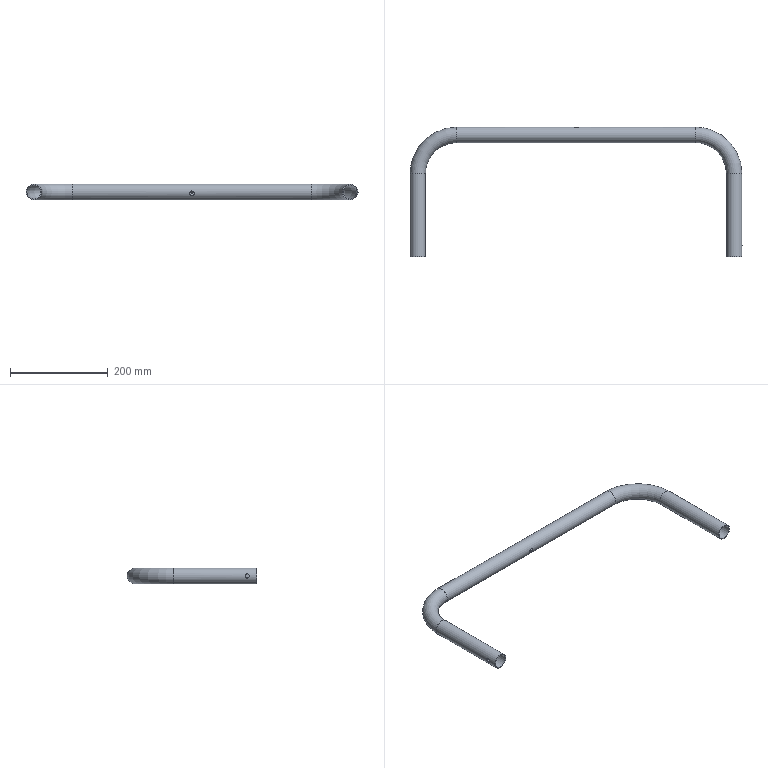Part | STEP file | 6151301 | 1 solid | 16 faces | box 679.8 x 265.9 x 31.8 mm | volume 153699 mm3 | cylinder 10 | torus 4 | plane 2 | commonest cylinder face diameters 28.8 x3 31.8 x3 8.5 x2 10 x2
STEP:
#1=CARTESIAN_POINT('',(0.,263.929,7.668));
#2=VERTEX_POINT('',#1);
#3=CARTESIAN_POINT('',(0.,263.929,7.668));
#4=CARTESIAN_POINT('',(-0.3326,263.929,7.668));
#5=CARTESIAN_POINT('',(-0.6592,263.946,7.638));
#6=CARTESIAN_POINT('',(-1.301,264.01,7.519));
#7=CARTESIAN_POINT('',(-1.62,264.058,7.429));
#8=CARTESIAN_POINT('',(-2.224,264.179,7.196));
#9=CARTESIAN_POINT('',(-2.51,264.251,7.053));
#10=CARTESIAN_POINT('',(-3.052,264.414,6.714));
#11=CARTESIAN_POINT('',(-3.307,264.505,6.518));
#12=CARTESIAN_POINT('',(-3.765,264.691,6.086));
#13=CARTESIAN_POINT('',(-3.971,264.787,5.85));
#14=CARTESIAN_POINT('',(-4.337,264.982,5.331));
#15=CARTESIAN_POINT('',(-4.491,265.078,5.056));
#16=CARTESIAN_POINT('',(-4.678,265.214,4.623));
#17=CARTESIAN_POINT('',(-4.734,265.258,4.475));
#18=CARTESIAN_POINT('',(-4.83,265.344,4.171));
#19=CARTESIAN_POINT('',(-4.871,265.386,4.015));
#20=CARTESIAN_POINT('',(-4.968,265.503,3.544));
#21=CARTESIAN_POINT('',(-5.,265.573,3.225));
#22=CARTESIAN_POINT('',(-5.,265.693,2.579));
#23=CARTESIAN_POINT('',(-4.967,265.743,2.249));
#24=CARTESIAN_POINT('',(-4.839,265.822,1.609));
#25=CARTESIAN_POINT('',(-4.744,265.85,1.297));
#26=CARTESIAN_POINT('',(-4.491,265.888,0.685));
#27=CARTESIAN_POINT('',(-4.335,265.898,0.3928));
#28=CARTESIAN_POINT('',(-3.974,265.902,-0.1551));
#29=CARTESIAN_POINT('',(-3.765,265.896,-0.4149));
#30=CARTESIAN_POINT('',(-3.304,265.877,-0.8872));
#31=CARTESIAN_POINT('',(-3.054,265.863,-1.099));
#32=CARTESIAN_POINT('',(-2.514,265.833,-1.472));
#33=CARTESIAN_POINT('',(-2.221,265.816,-1.635));
#34=CARTESIAN_POINT('',(-1.619,265.787,-1.895));
#35=CARTESIAN_POINT('',(-1.308,265.775,-1.995));
#36=CARTESIAN_POINT('',(-0.823,265.761,-2.096));
#37=CARTESIAN_POINT('',(-0.658,265.758,-2.122));
#38=CARTESIAN_POINT('',(-0.3299,265.753,-2.156));
#39=CARTESIAN_POINT('',(-0.166,265.752,-2.164));
#40=CARTESIAN_POINT('',(0.3255,265.752,-2.165));
#41=CARTESIAN_POINT('',(0.6546,265.757,-2.131));
#42=CARTESIAN_POINT('',(1.304,265.774,-1.996));
#43=CARTESIAN_POINT('',(1.616,265.787,-1.896));
#44=CARTESIAN_POINT('',(2.219,265.816,-1.636));
#45=CARTESIAN_POINT('',(2.512,265.833,-1.474));
#46=CARTESIAN_POINT('',(3.052,265.863,-1.1));
#47=CARTESIAN_POINT('',(3.303,265.877,-0.8884));
#48=CARTESIAN_POINT('',(3.765,265.896,-0.4156));
#49=CARTESIAN_POINT('',(3.973,265.902,-0.1564));
#50=CARTESIAN_POINT('',(4.334,265.898,0.3906));
#51=CARTESIAN_POINT('',(4.489,265.888,0.6818));
#52=CARTESIAN_POINT('',(4.743,265.85,1.294));
#53=CARTESIAN_POINT('',(4.838,265.822,1.607));
#54=CARTESIAN_POINT('',(4.934,265.764,2.085));
#55=CARTESIAN_POINT('',(4.959,265.741,2.246));
#56=CARTESIAN_POINT('',(4.992,265.692,2.571));
#57=CARTESIAN_POINT('',(5.,265.664,2.736));
#58=CARTESIAN_POINT('',(5.,265.574,3.222));
#59=CARTESIAN_POINT('',(4.968,265.504,3.541));
#60=CARTESIAN_POINT('',(4.839,265.347,4.168));
#61=CARTESIAN_POINT('',(4.742,265.26,4.476));
#62=CARTESIAN_POINT('',(4.491,265.078,5.055));
#63=CARTESIAN_POINT('',(4.337,264.983,5.33));
#64=CARTESIAN_POINT('',(3.972,264.788,5.849));
#65=CARTESIAN_POINT('',(3.765,264.691,6.086));
#66=CARTESIAN_POINT('',(3.307,264.505,6.518));
#67=CARTESIAN_POINT('',(3.052,264.414,6.714));
#68=CARTESIAN_POINT('',(2.511,264.252,7.053));
#69=CARTESIAN_POINT('',(2.225,264.179,7.195));
#70=CARTESIAN_POINT('',(1.621,264.059,7.429));
#71=CARTESIAN_POINT('',(1.302,264.01,7.519));
#72=CARTESIAN_POINT('',(0.6596,263.946,7.638));
#73=CARTESIAN_POINT('',(0.3326,263.929,7.668));
#74=CARTESIAN_POINT('',(0.,263.929,7.668));
#75=B_SPLINE_CURVE_WITH_KNOTS('',3,(#3,#4,#5,#6,#7,#8,#9,#10,#11,#12,#13,#14,#15,#16,#17,#18,#19,#20,#21,#22,#23,#24,#25,#26,#27,#28,#29,#30,#31,#32,#33,#34,#35,#36,#37,#38,#39,#40,#41,#42,#43,#44,#45,#46,#47,#48,#49,#50,#51,#52,#53,#54,#55,#56,#57,#58,#59,#60,#61,#62,#63,#64,#65,#66,#67,#68,#69,#70,#71,#72,#73,#74),.UNSPECIFIED.,.T.,.F.,(4,2,2,2,2,2,2,2,2,2,2,2,2,2,2,2,2,2,2,2,2,2,2,2,2,2,2,2,2,2,2,2,2,2,2,4),(0.,0.0009831,0.001966,0.002949,0.003933,0.004916,0.005899,0.00639,0.006882,0.007865,0.008848,0.009831,0.01081,0.0118,0.01278,0.01376,0.01475,0.01524,0.01573,0.01671,0.0177,0.01868,0.01966,0.02065,0.02163,0.02261,0.0231,0.0236,0.02458,0.02556,0.02654,0.02753,0.02851,0.02949,0.03048,0.03146),.UNSPECIFIED.);
#76=EDGE_CURVE('',#2,#2,#75,.T.);
#77=ORIENTED_EDGE('',*,*,#76,.T.);
#78=EDGE_LOOP('',(#77));
#79=FACE_BOUND('',#78,.T.);
#80=CARTESIAN_POINT('',(244.,250.,15.9));
#81=VERTEX_POINT('',#80);
#82=CARTESIAN_POINT('',(244.,250.,0.));
#83=DIRECTION('',(-1.,0.,0.));
#84=DIRECTION('',(0.,0.,1.));
#85=AXIS2_PLACEMENT_3D('',#82,#83,#84);
#86=CIRCLE('',#85,15.9);
#87=EDGE_CURVE('',#81,#81,#86,.T.);
#88=ORIENTED_EDGE('',*,*,#87,.T.);
#89=EDGE_LOOP('',(#88));
#90=FACE_OUTER_BOUND('',#89,.T.);
#91=CARTESIAN_POINT('',(-244.,250.,15.9));
#92=VERTEX_POINT('',#91);
#93=CARTESIAN_POINT('',(-244.,250.,0.));
#94=DIRECTION('',(-1.,0.,0.));
#95=DIRECTION('',(0.,0.,1.));
#96=AXIS2_PLACEMENT_3D('',#93,#94,#95);
#97=CIRCLE('',#96,15.9);
#98=EDGE_CURVE('',#92,#92,#97,.T.);
#99=ORIENTED_EDGE('',*,*,#98,.F.);
#100=EDGE_LOOP('',(#99));
#101=FACE_OUTER_BOUND('',#100,.T.);
#102=CARTESIAN_POINT('',(0.,234.248,2.167));
#103=VERTEX_POINT('',#102);
#104=CARTESIAN_POINT('',(0.,234.248,2.167));
#105=CARTESIAN_POINT('',(0.3326,234.248,2.167));
#106=CARTESIAN_POINT('',(0.6592,234.244,2.133));
#107=CARTESIAN_POINT('',(1.301,234.226,1.999));
#108=CARTESIAN_POINT('',(1.62,234.213,1.898));
#109=CARTESIAN_POINT('',(2.224,234.184,1.636));
#110=CARTESIAN_POINT('',(2.51,234.168,1.477));
#111=CARTESIAN_POINT('',(3.052,234.137,1.103));
#112=CARTESIAN_POINT('',(3.307,234.123,0.8869));
#113=CARTESIAN_POINT('',(3.765,234.104,0.4175));
#114=CARTESIAN_POINT('',(3.971,234.098,0.1619));
#115=CARTESIAN_POINT('',(4.337,234.102,-0.3926));
#116=CARTESIAN_POINT('',(4.491,234.112,-0.6832));
#117=CARTESIAN_POINT('',(4.678,234.14,-1.136));
#118=CARTESIAN_POINT('',(4.734,234.152,-1.29));
#119=CARTESIAN_POINT('',(4.83,234.18,-1.605));
#120=CARTESIAN_POINT('',(4.871,234.198,-1.766));
#121=CARTESIAN_POINT('',(4.968,234.256,-2.248));
#122=CARTESIAN_POINT('',(5.,234.306,-2.57));
#123=CARTESIAN_POINT('',(5.,234.425,-3.216));
#124=CARTESIAN_POINT('',(4.967,234.496,-3.542));
#125=CARTESIAN_POINT('',(4.839,234.652,-4.167));
#126=CARTESIAN_POINT('',(4.744,234.738,-4.47));
#127=CARTESIAN_POINT('',(4.491,234.922,-5.054));
#128=CARTESIAN_POINT('',(4.335,235.018,-5.33));
#129=CARTESIAN_POINT('',(3.974,235.21,-5.843));
#130=CARTESIAN_POINT('',(3.765,235.308,-6.084));
#131=CARTESIAN_POINT('',(3.304,235.495,-6.518));
#132=CARTESIAN_POINT('',(3.054,235.584,-6.711));
#133=CARTESIAN_POINT('',(2.514,235.746,-7.049));
#134=CARTESIAN_POINT('',(2.221,235.82,-7.195));
#135=CARTESIAN_POINT('',(1.619,235.941,-7.427));
#136=CARTESIAN_POINT('',(1.308,235.988,-7.515));
#137=CARTESIAN_POINT('',(0.823,236.037,-7.605));
#138=CARTESIAN_POINT('',(0.658,236.049,-7.628));
#139=CARTESIAN_POINT('',(0.3299,236.066,-7.658));
#140=CARTESIAN_POINT('',(0.166,236.07,-7.666));
#141=CARTESIAN_POINT('',(-0.3255,236.07,-7.666));
#142=CARTESIAN_POINT('',(-0.6546,236.054,-7.636));
#143=CARTESIAN_POINT('',(-1.304,235.989,-7.516));
#144=CARTESIAN_POINT('',(-1.616,235.941,-7.428));
#145=CARTESIAN_POINT('',(-2.219,235.821,-7.196));
#146=CARTESIAN_POINT('',(-2.512,235.747,-7.05));
#147=CARTESIAN_POINT('',(-3.052,235.585,-6.712));
#148=CARTESIAN_POINT('',(-3.303,235.496,-6.519));
#149=CARTESIAN_POINT('',(-3.765,235.308,-6.085));
#150=CARTESIAN_POINT('',(-3.973,235.211,-5.845));
#151=CARTESIAN_POINT('',(-4.334,235.018,-5.333));
#152=CARTESIAN_POINT('',(-4.489,234.923,-5.057));
#153=CARTESIAN_POINT('',(-4.743,234.739,-4.472));
#154=CARTESIAN_POINT('',(-4.838,234.653,-4.17));
#155=CARTESIAN_POINT('',(-4.934,234.536,-3.703));
#156=CARTESIAN_POINT('',(-4.959,234.499,-3.544));
#157=CARTESIAN_POINT('',(-4.992,234.429,-3.223));
#158=CARTESIAN_POINT('',(-5.,234.396,-3.059));
#159=CARTESIAN_POINT('',(-5.,234.306,-2.573));
#160=CARTESIAN_POINT('',(-4.968,234.257,-2.251));
#161=CARTESIAN_POINT('',(-4.839,234.178,-1.609));
#162=CARTESIAN_POINT('',(-4.742,234.15,-1.29));
#163=CARTESIAN_POINT('',(-4.491,234.112,-0.6845));
#164=CARTESIAN_POINT('',(-4.337,234.102,-0.3932));
#165=CARTESIAN_POINT('',(-3.972,234.098,0.1612));
#166=CARTESIAN_POINT('',(-3.765,234.104,0.4169));
#167=CARTESIAN_POINT('',(-3.307,234.123,0.8867));
#168=CARTESIAN_POINT('',(-3.052,234.137,1.103));
#169=CARTESIAN_POINT('',(-2.511,234.168,1.477));
#170=CARTESIAN_POINT('',(-2.225,234.184,1.636));
#171=CARTESIAN_POINT('',(-1.621,234.213,1.897));
#172=CARTESIAN_POINT('',(-1.302,234.226,1.999));
#173=CARTESIAN_POINT('',(-0.6596,234.244,2.133));
#174=CARTESIAN_POINT('',(-0.3326,234.248,2.167));
#175=CARTESIAN_POINT('',(0.,234.248,2.167));
#176=B_SPLINE_CURVE_WITH_KNOTS('',3,(#104,#105,#106,#107,#108,#109,#110,#111,#112,#113,#114,#115,#116,#117,#118,#119,#120,#121,#122,#123,#124,#125,#126,#127,#128,#129,#130,#131,#132,#133,#134,#135,#136,#137,#138,#139,#140,#141,#142,#143,#144,#145,#146,#147,#148,#149,#150,#151,#152,#153,#154,#155,#156,#157,#158,#159,#160,#161,#162,#163,#164,#165,#166,#167,#168,#169,#170,#171,#172,#173,#174,#175),.UNSPECIFIED.,.T.,.F.,(4,2,2,2,2,2,2,2,2,2,2,2,2,2,2,2,2,2,2,2,2,2,2,2,2,2,2,2,2,2,2,2,2,2,2,4),(0.,0.0009831,0.001966,0.002949,0.003933,0.004916,0.005899,0.00639,0.006882,0.007865,0.008848,0.009831,0.01081,0.0118,0.01278,0.01376,0.01475,0.01524,0.01573,0.01671,0.0177,0.01868,0.01966,0.02065,0.02163,0.02261,0.0231,0.0236,0.02458,0.02556,0.02654,0.02753,0.02851,0.02949,0.03048,0.03146),.UNSPECIFIED.);
#177=EDGE_CURVE('',#103,#103,#176,.T.);
#178=ORIENTED_EDGE('',*,*,#177,.T.);
#179=EDGE_LOOP('',(#178));
#180=FACE_BOUND('',#179,.T.);
#181=CARTESIAN_POINT('',(244.,250.,0.));
#182=DIRECTION('',(-1.,0.,0.));
#183=DIRECTION('',(0.,0.,1.));
#184=AXIS2_PLACEMENT_3D('',#181,#182,#183);
#185=CYLINDRICAL_SURFACE('',#184,15.9);
#186=ADVANCED_FACE('',(#79,#90,#101,#180),#185,.T.);
#187=CARTESIAN_POINT('',(0.,262.366,7.378));
#188=VERTEX_POINT('',#187);
#189=CARTESIAN_POINT('',(0.,262.366,7.378));
#190=CARTESIAN_POINT('',(-0.3331,262.366,7.378));
#191=CARTESIAN_POINT('',(-0.6602,262.384,7.348));
#192=CARTESIAN_POINT('',(-1.303,262.453,7.23));
#193=CARTESIAN_POINT('',(-1.621,262.505,7.141));
#194=CARTESIAN_POINT('',(-2.226,262.635,6.909));
#195=CARTESIAN_POINT('',(-2.512,262.712,6.767));
#196=CARTESIAN_POINT('',(-3.053,262.886,6.43));
#197=CARTESIAN_POINT('',(-3.307,262.982,6.235));
#198=CARTESIAN_POINT('',(-3.764,263.179,5.807));
#199=CARTESIAN_POINT('',(-3.971,263.281,5.571));
#200=CARTESIAN_POINT('',(-4.336,263.487,5.054));
#201=CARTESIAN_POINT('',(-4.49,263.586,4.781));
#202=CARTESIAN_POINT('',(-4.678,263.728,4.349));
#203=CARTESIAN_POINT('',(-4.733,263.774,4.202));
#204=CARTESIAN_POINT('',(-4.829,263.863,3.898));
#205=CARTESIAN_POINT('',(-4.87,263.906,3.742));
#206=CARTESIAN_POINT('',(-4.967,264.027,3.271));
#207=CARTESIAN_POINT('',(-5.,264.098,2.952));
#208=CARTESIAN_POINT('',(-5.,264.218,2.305));
#209=CARTESIAN_POINT('',(-4.967,264.268,1.974));
#210=CARTESIAN_POINT('',(-4.838,264.342,1.334));
#211=CARTESIAN_POINT('',(-4.743,264.367,1.02));
#212=CARTESIAN_POINT('',(-4.489,264.398,0.4061));
#213=CARTESIAN_POINT('',(-4.334,264.402,0.114));
#214=CARTESIAN_POINT('',(-3.973,264.396,-0.4354));
#215=CARTESIAN_POINT('',(-3.764,264.385,-0.6962));
#216=CARTESIAN_POINT('',(-3.304,264.354,-1.169));
#217=CARTESIAN_POINT('',(-3.054,264.335,-1.382));
#218=CARTESIAN_POINT('',(-2.515,264.294,-1.757));
#219=CARTESIAN_POINT('',(-2.222,264.272,-1.921));
#220=CARTESIAN_POINT('',(-1.621,264.234,-2.183));
#221=CARTESIAN_POINT('',(-1.309,264.218,-2.283));
#222=CARTESIAN_POINT('',(-0.8233,264.201,-2.385));
#223=CARTESIAN_POINT('',(-0.6582,264.197,-2.411));
#224=CARTESIAN_POINT('',(-0.3301,264.191,-2.446));
#225=CARTESIAN_POINT('',(-0.001961,264.188,-2.463));
#226=CARTESIAN_POINT('',(0.3261,264.191,-2.446));
#227=CARTESIAN_POINT('',(0.6541,264.197,-2.412));
#228=CARTESIAN_POINT('',(0.819,264.201,-2.386));
#229=CARTESIAN_POINT('',(1.306,264.218,-2.284));
#230=CARTESIAN_POINT('',(1.618,264.234,-2.184));
#231=CARTESIAN_POINT('',(2.222,264.272,-1.921));
#232=CARTESIAN_POINT('',(2.514,264.294,-1.758));
#233=CARTESIAN_POINT('',(3.053,264.335,-1.383));
#234=CARTESIAN_POINT('',(3.304,264.354,-1.17));
#235=CARTESIAN_POINT('',(3.766,264.385,-0.6944));
#236=CARTESIAN_POINT('',(3.973,264.396,-0.4358));
#237=CARTESIAN_POINT('',(4.333,264.402,0.1125));
#238=CARTESIAN_POINT('',(4.489,264.398,0.4062));
#239=CARTESIAN_POINT('',(4.742,264.367,1.018));
#240=CARTESIAN_POINT('',(4.838,264.342,1.331));
#241=CARTESIAN_POINT('',(4.967,264.268,1.971));
#242=CARTESIAN_POINT('',(5.,264.219,2.302));
#243=CARTESIAN_POINT('',(5.,264.099,2.95));
#244=CARTESIAN_POINT('',(4.968,264.028,3.269));
#245=CARTESIAN_POINT('',(4.871,263.907,3.74));
#246=CARTESIAN_POINT('',(4.83,263.864,3.896));
#247=CARTESIAN_POINT('',(4.734,263.775,4.2));
#248=CARTESIAN_POINT('',(4.678,263.729,4.348));
#249=CARTESIAN_POINT('',(4.49,263.587,4.781));
#250=CARTESIAN_POINT('',(4.335,263.486,5.057));
#251=CARTESIAN_POINT('',(3.97,263.281,5.572));
#252=CARTESIAN_POINT('',(3.764,263.179,5.807));
#253=CARTESIAN_POINT('',(3.306,262.982,6.237));
#254=CARTESIAN_POINT('',(3.05,262.885,6.432));
#255=CARTESIAN_POINT('',(2.511,262.712,6.767));
#256=CARTESIAN_POINT('',(2.225,262.635,6.909));
#257=CARTESIAN_POINT('',(1.771,262.538,7.083));
#258=CARTESIAN_POINT('',(1.615,262.508,7.135));
#259=CARTESIAN_POINT('',(1.3,262.458,7.223));
#260=CARTESIAN_POINT('',(1.141,262.436,7.26));
#261=CARTESIAN_POINT('',(0.6602,262.384,7.348));
#262=CARTESIAN_POINT('',(0.3331,262.366,7.378));
#263=CARTESIAN_POINT('',(0.,262.366,7.378));
#264=B_SPLINE_CURVE_WITH_KNOTS('',3,(#189,#190,#191,#192,#193,#194,#195,#196,#197,#198,#199,#200,#201,#202,#203,#204,#205,#206,#207,#208,#209,#210,#211,#212,#213,#214,#215,#216,#217,#218,#219,#220,#221,#222,#223,#224,#225,#226,#227,#228,#229,#230,#231,#232,#233,#234,#235,#236,#237,#238,#239,#240,#241,#242,#243,#244,#245,#246,#247,#248,#249,#250,#251,#252,#253,#254,#255,#256,#257,#258,#259,#260,#261,#262,#263),.UNSPECIFIED.,.T.,.F.,(4,2,2,2,2,2,2,2,2,2,2,2,2,2,2,2,2,2,1,2,2,2,2,2,2,2,2,2,2,2,2,2,2,2,2,2,2,4),(0.,0.0009846,0.001969,0.002954,0.003938,0.004923,0.005908,0.0064,0.006892,0.007877,0.008861,0.009846,0.01083,0.01182,0.0128,0.01378,0.01477,0.01526,0.01575,0.01625,0.01674,0.01772,0.01871,0.01969,0.02068,0.02166,0.02265,0.02363,0.02461,0.02511,0.0256,0.02658,0.02757,0.02855,0.02954,0.03003,0.03052,0.03151),.UNSPECIFIED.);
#265=EDGE_CURVE('',#188,#188,#264,.T.);
#266=ORIENTED_EDGE('',*,*,#265,.F.);
#267=EDGE_LOOP('',(#266));
#268=FACE_BOUND('',#267,.T.);
#269=CARTESIAN_POINT('',(244.,250.,14.4));
#270=VERTEX_POINT('',#269);
#271=CARTESIAN_POINT('',(244.,250.,0.));
#272=DIRECTION('',(-1.,0.,0.));
#273=DIRECTION('',(0.,0.,1.));
#274=AXIS2_PLACEMENT_3D('',#271,#272,#273);
#275=CIRCLE('',#274,14.4);
#276=EDGE_CURVE('',#270,#270,#275,.T.);
#277=ORIENTED_EDGE('',*,*,#276,.F.);
#278=EDGE_LOOP('',(#277));
#279=FACE_OUTER_BOUND('',#278,.T.);
#280=CARTESIAN_POINT('',(-244.,250.,14.4));
#281=VERTEX_POINT('',#280);
#282=CARTESIAN_POINT('',(-244.,250.,0.));
#283=DIRECTION('',(-1.,0.,0.));
#284=DIRECTION('',(0.,0.,1.));
#285=AXIS2_PLACEMENT_3D('',#282,#283,#284);
#286=CIRCLE('',#285,14.4);
#287=EDGE_CURVE('',#281,#281,#286,.T.);
#288=ORIENTED_EDGE('',*,*,#287,.T.);
#289=EDGE_LOOP('',(#288));
#290=FACE_OUTER_BOUND('',#289,.T.);
#291=CARTESIAN_POINT('',(0.,235.811,2.457));
#292=VERTEX_POINT('',#291);
#293=CARTESIAN_POINT('',(0.,235.811,2.457));
#294=CARTESIAN_POINT('',(0.3331,235.811,2.457));
#295=CARTESIAN_POINT('',(0.6602,235.805,2.422));
#296=CARTESIAN_POINT('',(1.303,235.783,2.287));
#297=CARTESIAN_POINT('',(1.621,235.766,2.185));
#298=CARTESIAN_POINT('',(2.226,235.728,1.922));
#299=CARTESIAN_POINT('',(2.512,235.707,1.762));
#300=CARTESIAN_POINT('',(3.053,235.666,1.385));
#301=CARTESIAN_POINT('',(3.307,235.646,1.169));
#302=CARTESIAN_POINT('',(3.764,235.615,0.6981));
#303=CARTESIAN_POINT('',(3.971,235.604,0.4417));
#304=CARTESIAN_POINT('',(4.336,235.598,-0.1145));
#305=CARTESIAN_POINT('',(4.49,235.603,-0.4052));
#306=CARTESIAN_POINT('',(4.678,235.625,-0.8593));
#307=CARTESIAN_POINT('',(4.733,235.635,-1.014));
#308=CARTESIAN_POINT('',(4.829,235.661,-1.329));
#309=CARTESIAN_POINT('',(4.87,235.676,-1.49));
#310=CARTESIAN_POINT('',(4.967,235.732,-1.973));
#311=CARTESIAN_POINT('',(5.,235.78,-2.296));
#312=CARTESIAN_POINT('',(5.,235.9,-2.943));
#313=CARTESIAN_POINT('',(4.967,235.972,-3.27));
#314=CARTESIAN_POINT('',(4.838,236.133,-3.895));
#315=CARTESIAN_POINT('',(4.743,236.222,-4.197));
#316=CARTESIAN_POINT('',(4.489,236.413,-4.78));
#317=CARTESIAN_POINT('',(4.334,236.514,-5.055));
#318=CARTESIAN_POINT('',(3.973,236.716,-5.566));
#319=CARTESIAN_POINT('',(3.764,236.82,-5.805));
#320=CARTESIAN_POINT('',(3.304,237.018,-6.236));
#321=CARTESIAN_POINT('',(3.054,237.112,-6.427));
#322=CARTESIAN_POINT('',(2.515,237.286,-6.763));
#323=CARTESIAN_POINT('',(2.222,237.364,-6.908));
#324=CARTESIAN_POINT('',(1.621,237.493,-7.139));
#325=CARTESIAN_POINT('',(1.309,237.544,-7.227));
#326=CARTESIAN_POINT('',(0.8233,237.597,-7.316));
#327=CARTESIAN_POINT('',(0.6582,237.61,-7.339));
#328=CARTESIAN_POINT('',(0.3301,237.628,-7.369));
#329=CARTESIAN_POINT('',(0.001961,237.637,-7.383));
#330=CARTESIAN_POINT('',(-0.3261,237.628,-7.369));
#331=CARTESIAN_POINT('',(-0.6541,237.611,-7.339));
#332=CARTESIAN_POINT('',(-0.819,237.597,-7.317));
#333=CARTESIAN_POINT('',(-1.306,237.545,-7.227));
#334=CARTESIAN_POINT('',(-1.618,237.494,-7.14));
#335=CARTESIAN_POINT('',(-2.222,237.365,-6.908));
#336=CARTESIAN_POINT('',(-2.514,237.286,-6.763));
#337=CARTESIAN_POINT('',(-3.053,237.113,-6.428));
#338=CARTESIAN_POINT('',(-3.304,237.018,-6.236));
#339=CARTESIAN_POINT('',(-3.766,236.819,-5.803));
#340=CARTESIAN_POINT('',(-3.973,236.716,-5.566));
#341=CARTESIAN_POINT('',(-4.333,236.514,-5.056));
#342=CARTESIAN_POINT('',(-4.489,236.413,-4.78));
#343=CARTESIAN_POINT('',(-4.742,236.222,-4.198));
#344=CARTESIAN_POINT('',(-4.838,236.134,-3.897));
#345=CARTESIAN_POINT('',(-4.967,235.973,-3.273));
#346=CARTESIAN_POINT('',(-5.,235.901,-2.947));
#347=CARTESIAN_POINT('',(-5.,235.781,-2.299));
#348=CARTESIAN_POINT('',(-4.968,235.732,-1.976));
#349=CARTESIAN_POINT('',(-4.871,235.677,-1.492));
#350=CARTESIAN_POINT('',(-4.83,235.661,-1.331));
#351=CARTESIAN_POINT('',(-4.734,235.635,-1.015));
#352=CARTESIAN_POINT('',(-4.678,235.625,-0.8607));
#353=CARTESIAN_POINT('',(-4.49,235.603,-0.4055));
#354=CARTESIAN_POINT('',(-4.335,235.598,-0.1115));
#355=CARTESIAN_POINT('',(-3.97,235.604,0.4423));
#356=CARTESIAN_POINT('',(-3.764,235.615,0.6985));
#357=CARTESIAN_POINT('',(-3.306,235.646,1.17));
#358=CARTESIAN_POINT('',(-3.05,235.666,1.387));
#359=CARTESIAN_POINT('',(-2.511,235.707,1.762));
#360=CARTESIAN_POINT('',(-2.225,235.728,1.922));
#361=CARTESIAN_POINT('',(-1.771,235.757,2.12));
#362=CARTESIAN_POINT('',(-1.615,235.766,2.178));
#363=CARTESIAN_POINT('',(-1.3,235.781,2.279));
#364=CARTESIAN_POINT('',(-1.141,235.788,2.321));
#365=CARTESIAN_POINT('',(-0.6602,235.805,2.422));
#366=CARTESIAN_POINT('',(-0.3331,235.811,2.457));
#367=CARTESIAN_POINT('',(0.,235.811,2.457));
#368=B_SPLINE_CURVE_WITH_KNOTS('',3,(#293,#294,#295,#296,#297,#298,#299,#300,#301,#302,#303,#304,#305,#306,#307,#308,#309,#310,#311,#312,#313,#314,#315,#316,#317,#318,#319,#320,#321,#322,#323,#324,#325,#326,#327,#328,#329,#330,#331,#332,#333,#334,#335,#336,#337,#338,#339,#340,#341,#342,#343,#344,#345,#346,#347,#348,#349,#350,#351,#352,#353,#354,#355,#356,#357,#358,#359,#360,#361,#362,#363,#364,#365,#366,#367),.UNSPECIFIED.,.T.,.F.,(4,2,2,2,2,2,2,2,2,2,2,2,2,2,2,2,2,2,1,2,2,2,2,2,2,2,2,2,2,2,2,2,2,2,2,2,2,4),(0.,0.0009846,0.001969,0.002954,0.003938,0.004923,0.005908,0.0064,0.006892,0.007877,0.008861,0.009846,0.01083,0.01182,0.0128,0.01378,0.01477,0.01526,0.01575,0.01625,0.01674,0.01772,0.01871,0.01969,0.02068,0.02166,0.02265,0.02363,0.02461,0.02511,0.0256,0.02658,0.02757,0.02855,0.02954,0.03003,0.03052,0.03151),.UNSPECIFIED.);
#369=EDGE_CURVE('',#292,#292,#368,.T.);
#370=ORIENTED_EDGE('',*,*,#369,.F.);
#371=EDGE_LOOP('',(#370));
#372=FACE_BOUND('',#371,.T.);
#373=CARTESIAN_POINT('',(244.,250.,0.));
#374=DIRECTION('',(-1.,0.,0.));
#375=DIRECTION('',(0.,0.,1.));
#376=AXIS2_PLACEMENT_3D('',#373,#374,#375);
#377=CYLINDRICAL_SURFACE('',#376,14.4);
#378=ADVANCED_FACE('',(#268,#279,#290,#372),#377,.F.);
#379=CARTESIAN_POINT('',(-324.,0.,15.9));
#380=VERTEX_POINT('',#379);
#381=CARTESIAN_POINT('',(-324.,0.,0.));
#382=DIRECTION('',(0.,-1.,0.));
#383=DIRECTION('',(0.,0.,1.));
#384=AXIS2_PLACEMENT_3D('',#381,#382,#383);
#385=CIRCLE('',#384,15.9);
#386=EDGE_CURVE('',#380,#380,#385,.T.);
#387=ORIENTED_EDGE('',*,*,#386,.F.);
#388=EDGE_LOOP('',(#387));
#389=FACE_OUTER_BOUND('',#388,.T.);
#390=CARTESIAN_POINT('',(-324.,170.,15.9));
#391=VERTEX_POINT('',#390);
#392=CARTESIAN_POINT('',(-324.,170.,0.));
#393=DIRECTION('',(0.,-1.,0.));
#394=DIRECTION('',(0.,0.,1.));
#395=AXIS2_PLACEMENT_3D('',#392,#393,#394);
#396=CIRCLE('',#395,15.9);
#397=EDGE_CURVE('',#391,#391,#396,.T.);
#398=ORIENTED_EDGE('',*,*,#397,.T.);
#399=EDGE_LOOP('',(#398));
#400=FACE_OUTER_BOUND('',#399,.T.);
#401=CARTESIAN_POINT('',(-339.321,20.,4.25));
#402=VERTEX_POINT('',#401);
#403=CARTESIAN_POINT('',(-339.321,20.,4.25));
#404=CARTESIAN_POINT('',(-339.321,19.718,4.25));
#405=CARTESIAN_POINT('',(-339.329,19.441,4.222));
#406=CARTESIAN_POINT('',(-339.359,18.896,4.113));
#407=CARTESIAN_POINT('',(-339.381,18.625,4.031));
#408=CARTESIAN_POINT('',(-339.435,18.111,3.817));
#409=CARTESIAN_POINT('',(-339.467,17.868,3.687));
#410=CARTESIAN_POINT('',(-339.538,17.407,3.378));
#411=CARTESIAN_POINT('',(-339.576,17.189,3.2));
#412=CARTESIAN_POINT('',(-339.651,16.799,2.81));
#413=CARTESIAN_POINT('',(-339.688,16.624,2.597));
#414=CARTESIAN_POINT('',(-339.758,16.313,2.133));
#415=CARTESIAN_POINT('',(-339.79,16.182,1.887));
#416=CARTESIAN_POINT('',(-339.842,15.97,1.376));
#417=CARTESIAN_POINT('',(-339.864,15.887,1.107));
#418=CARTESIAN_POINT('',(-339.893,15.777,0.5579));
#419=CARTESIAN_POINT('',(-339.9,15.75,0.2813));
#420=CARTESIAN_POINT('',(-339.9,15.75,-0.2759));
#421=CARTESIAN_POINT('',(-339.893,15.778,-0.559));
#422=CARTESIAN_POINT('',(-339.864,15.887,-1.105));
#423=CARTESIAN_POINT('',(-339.843,15.967,-1.371));
#424=CARTESIAN_POINT('',(-339.763,16.289,-2.145));
#425=CARTESIAN_POINT('',(-339.689,16.602,-2.612));
#426=CARTESIAN_POINT('',(-339.576,17.192,-3.202));
#427=CARTESIAN_POINT('',(-339.538,17.405,-3.377));
#428=CARTESIAN_POINT('',(-339.468,17.864,-3.685));
#429=CARTESIAN_POINT('',(-339.435,18.113,-3.818));
#430=CARTESIAN_POINT('',(-339.381,18.625,-4.031));
#431=CARTESIAN_POINT('',(-339.359,18.89,-4.112));
#432=CARTESIAN_POINT('',(-339.329,19.438,-4.222));
#433=CARTESIAN_POINT('',(-339.322,19.72,-4.25));
#434=CARTESIAN_POINT('',(-339.321,20.276,-4.25));
#435=CARTESIAN_POINT('',(-339.329,20.554,-4.223));
#436=CARTESIAN_POINT('',(-339.359,21.106,-4.113));
#437=CARTESIAN_POINT('',(-339.381,21.372,-4.032));
#438=CARTESIAN_POINT('',(-339.435,21.884,-3.82));
#439=CARTESIAN_POINT('',(-339.468,22.133,-3.687));
#440=CARTESIAN_POINT('',(-339.538,22.594,-3.378));
#441=CARTESIAN_POINT('',(-339.575,22.807,-3.203));
#442=CARTESIAN_POINT('',(-339.651,23.199,-2.812));
#443=CARTESIAN_POINT('',(-339.689,23.377,-2.595));
#444=CARTESIAN_POINT('',(-339.758,23.685,-2.136));
#445=CARTESIAN_POINT('',(-339.789,23.816,-1.892));
#446=CARTESIAN_POINT('',(-339.843,24.031,-1.375));
#447=CARTESIAN_POINT('',(-339.864,24.112,-1.108));
#448=CARTESIAN_POINT('',(-339.892,24.222,-0.5634));
#449=CARTESIAN_POINT('',(-339.9,24.25,-0.2821));
#450=CARTESIAN_POINT('',(-339.9,24.25,0.2784));
#451=CARTESIAN_POINT('',(-339.893,24.223,0.5551));
#452=CARTESIAN_POINT('',(-339.864,24.114,1.102));
#453=CARTESIAN_POINT('',(-339.843,24.032,1.373));
#454=CARTESIAN_POINT('',(-339.79,23.819,1.886));
#455=CARTESIAN_POINT('',(-339.758,23.688,2.13));
#456=CARTESIAN_POINT('',(-339.689,23.378,2.594));
#457=CARTESIAN_POINT('',(-339.651,23.202,2.809));
#458=CARTESIAN_POINT('',(-339.576,22.812,3.199));
#459=CARTESIAN_POINT('',(-339.538,22.596,3.376));
#460=CARTESIAN_POINT('',(-339.468,22.134,3.686));
#461=CARTESIAN_POINT('',(-339.436,21.89,3.817));
#462=CARTESIAN_POINT('',(-339.381,21.378,4.03));
#463=CARTESIAN_POINT('',(-339.359,21.107,4.113));
#464=CARTESIAN_POINT('',(-339.329,20.56,4.222));
#465=CARTESIAN_POINT('',(-339.321,20.282,4.25));
#466=CARTESIAN_POINT('',(-339.321,20.,4.25));
#467=B_SPLINE_CURVE_WITH_KNOTS('',3,(#403,#404,#405,#406,#407,#408,#409,#410,#411,#412,#413,#414,#415,#416,#417,#418,#419,#420,#421,#422,#423,#424,#425,#426,#427,#428,#429,#430,#431,#432,#433,#434,#435,#436,#437,#438,#439,#440,#441,#442,#443,#444,#445,#446,#447,#448,#449,#450,#451,#452,#453,#454,#455,#456,#457,#458,#459,#460,#461,#462,#463,#464,#465,#466),.UNSPECIFIED.,.T.,.F.,(4,2,2,2,2,2,2,2,2,2,2,2,2,2,2,2,2,2,2,2,2,2,2,2,2,2,2,2,2,2,2,4),(0.,0.0008342,0.001668,0.002502,0.003337,0.004171,0.005005,0.005839,0.006673,0.007507,0.008342,0.01001,0.01084,0.01168,0.01251,0.01335,0.01418,0.01501,0.01585,0.01668,0.01752,0.01835,0.01919,0.02002,0.02085,0.02169,0.02252,0.02336,0.02419,0.02502,0.02586,0.02669),.UNSPECIFIED.);
#468=EDGE_CURVE('',#402,#402,#467,.T.);
#469=ORIENTED_EDGE('',*,*,#468,.T.);
#470=EDGE_LOOP('',(#469));
#471=FACE_BOUND('',#470,.T.);
#472=CARTESIAN_POINT('',(-324.,170.,0.));
#473=DIRECTION('',(0.,-1.,0.));
#474=DIRECTION('',(1.,0.,0.));
#475=AXIS2_PLACEMENT_3D('',#472,#473,#474);
#476=CYLINDRICAL_SURFACE('',#475,15.9);
#477=ADVANCED_FACE('',(#389,#400,#471),#476,.T.);
#478=CARTESIAN_POINT('',(-324.,0.,14.4));
#479=VERTEX_POINT('',#478);
#480=CARTESIAN_POINT('',(-324.,0.,0.));
#481=DIRECTION('',(0.,-1.,0.));
#482=DIRECTION('',(0.,0.,1.));
#483=AXIS2_PLACEMENT_3D('',#480,#481,#482);
#484=CIRCLE('',#483,14.4);
#485=EDGE_CURVE('',#479,#479,#484,.T.);
#486=ORIENTED_EDGE('',*,*,#485,.T.);
#487=EDGE_LOOP('',(#486));
#488=FACE_OUTER_BOUND('',#487,.T.);
#489=CARTESIAN_POINT('',(-324.,170.,14.4));
#490=VERTEX_POINT('',#489);
#491=CARTESIAN_POINT('',(-324.,170.,0.));
#492=DIRECTION('',(0.,-1.,0.));
#493=DIRECTION('',(0.,0.,1.));
#494=AXIS2_PLACEMENT_3D('',#491,#492,#493);
#495=CIRCLE('',#494,14.4);
#496=EDGE_CURVE('',#490,#490,#495,.T.);
#497=ORIENTED_EDGE('',*,*,#496,.F.);
#498=EDGE_LOOP('',(#497));
#499=FACE_OUTER_BOUND('',#498,.T.);
#500=CARTESIAN_POINT('',(-337.759,20.,4.25));
#501=VERTEX_POINT('',#500);
#502=CARTESIAN_POINT('',(-337.759,20.,4.25));
#503=CARTESIAN_POINT('',(-337.759,19.718,4.25));
#504=CARTESIAN_POINT('',(-337.767,19.44,4.222));
#505=CARTESIAN_POINT('',(-337.8,18.895,4.113));
#506=CARTESIAN_POINT('',(-337.825,18.624,4.031));
#507=CARTESIAN_POINT('',(-337.885,18.11,3.817));
#508=CARTESIAN_POINT('',(-337.921,17.867,3.686));
#509=CARTESIAN_POINT('',(-337.999,17.406,3.378));
#510=CARTESIAN_POINT('',(-338.041,17.189,3.2));
#511=CARTESIAN_POINT('',(-338.125,16.8,2.81));
#512=CARTESIAN_POINT('',(-338.166,16.624,2.597));
#513=CARTESIAN_POINT('',(-338.243,16.313,2.133));
#514=CARTESIAN_POINT('',(-338.278,16.182,1.888));
#515=CARTESIAN_POINT('',(-338.336,15.97,1.377));
#516=CARTESIAN_POINT('',(-338.36,15.887,1.108));
#517=CARTESIAN_POINT('',(-338.392,15.778,0.5585));
#518=CARTESIAN_POINT('',(-338.4,15.75,0.2817));
#519=CARTESIAN_POINT('',(-338.4,15.75,-0.2762));
#520=CARTESIAN_POINT('',(-338.392,15.778,-0.5596));
#521=CARTESIAN_POINT('',(-338.36,15.887,-1.106));
#522=CARTESIAN_POINT('',(-338.337,15.968,-1.372));
#523=CARTESIAN_POINT('',(-338.278,16.182,-1.888));
#524=CARTESIAN_POINT('',(-338.243,16.315,-2.135));
#525=CARTESIAN_POINT('',(-338.166,16.622,-2.593));
#526=CARTESIAN_POINT('',(-338.125,16.799,-2.81));
#527=CARTESIAN_POINT('',(-338.041,17.192,-3.202));
#528=CARTESIAN_POINT('',(-337.999,17.404,-3.377));
#529=CARTESIAN_POINT('',(-337.922,17.863,-3.684));
#530=CARTESIAN_POINT('',(-337.885,18.112,-3.818));
#531=CARTESIAN_POINT('',(-337.825,18.624,-4.031));
#532=CARTESIAN_POINT('',(-337.801,18.889,-4.112));
#533=CARTESIAN_POINT('',(-337.767,19.438,-4.222));
#534=CARTESIAN_POINT('',(-337.759,19.72,-4.25));
#535=CARTESIAN_POINT('',(-337.759,20.276,-4.25));
#536=CARTESIAN_POINT('',(-337.767,20.555,-4.223));
#537=CARTESIAN_POINT('',(-337.8,21.107,-4.113));
#538=CARTESIAN_POINT('',(-337.825,21.373,-4.032));
#539=CARTESIAN_POINT('',(-337.885,21.885,-3.819));
#540=CARTESIAN_POINT('',(-337.921,22.134,-3.686));
#541=CARTESIAN_POINT('',(-337.999,22.594,-3.378));
#542=CARTESIAN_POINT('',(-338.041,22.807,-3.203));
#543=CARTESIAN_POINT('',(-338.124,23.2,-2.811));
#544=CARTESIAN_POINT('',(-338.166,23.377,-2.595));
#545=CARTESIAN_POINT('',(-338.243,23.684,-2.137));
#546=CARTESIAN_POINT('',(-338.277,23.816,-1.893));
#547=CARTESIAN_POINT('',(-338.337,24.031,-1.374));
#548=CARTESIAN_POINT('',(-338.36,24.112,-1.108));
#549=CARTESIAN_POINT('',(-338.392,24.222,-0.5637));
#550=CARTESIAN_POINT('',(-338.4,24.25,-0.2814));
#551=CARTESIAN_POINT('',(-338.4,24.25,0.2789));
#552=CARTESIAN_POINT('',(-338.392,24.223,0.5558));
#553=CARTESIAN_POINT('',(-338.36,24.114,1.103));
#554=CARTESIAN_POINT('',(-338.337,24.031,1.375));
#555=CARTESIAN_POINT('',(-338.278,23.818,1.887));
#556=CARTESIAN_POINT('',(-338.243,23.688,2.131));
#557=CARTESIAN_POINT('',(-338.166,23.377,2.596));
#558=CARTESIAN_POINT('',(-338.125,23.201,2.809));
#559=CARTESIAN_POINT('',(-338.042,22.812,3.199));
#560=CARTESIAN_POINT('',(-337.999,22.595,3.377));
#561=CARTESIAN_POINT('',(-337.921,22.134,3.686));
#562=CARTESIAN_POINT('',(-337.886,21.891,3.816));
#563=CARTESIAN_POINT('',(-337.825,21.378,4.03));
#564=CARTESIAN_POINT('',(-337.8,21.107,4.113));
#565=CARTESIAN_POINT('',(-337.767,20.56,4.222));
#566=CARTESIAN_POINT('',(-337.759,20.282,4.25));
#567=CARTESIAN_POINT('',(-337.759,20.,4.25));
#568=B_SPLINE_CURVE_WITH_KNOTS('',3,(#502,#503,#504,#505,#506,#507,#508,#509,#510,#511,#512,#513,#514,#515,#516,#517,#518,#519,#520,#521,#522,#523,#524,#525,#526,#527,#528,#529,#530,#531,#532,#533,#534,#535,#536,#537,#538,#539,#540,#541,#542,#543,#544,#545,#546,#547,#548,#549,#550,#551,#552,#553,#554,#555,#556,#557,#558,#559,#560,#561,#562,#563,#564,#565,#566,#567),.UNSPECIFIED.,.T.,.F.,(4,2,2,2,2,2,2,2,2,2,2,2,2,2,2,2,2,2,2,2,2,2,2,2,2,2,2,2,2,2,2,2,4),(0.,0.000835,0.00167,0.002505,0.00334,0.004175,0.00501,0.005845,0.00668,0.007515,0.00835,0.009185,0.01002,0.01086,0.01169,0.01253,0.01336,0.0142,0.01503,0.01587,0.0167,0.01754,0.01837,0.01921,0.02004,0.02088,0.02171,0.02255,0.02338,0.02422,0.02505,0.02589,0.02672),.UNSPECIFIED.);
#569=EDGE_CURVE('',#501,#501,#568,.T.);
#570=ORIENTED_EDGE('',*,*,#569,.F.);
#571=EDGE_LOOP('',(#570));
#572=FACE_BOUND('',#571,.T.);
#573=CARTESIAN_POINT('',(-324.,170.,0.));
#574=DIRECTION('',(0.,-1.,0.));
#575=DIRECTION('',(1.,0.,0.));
#576=AXIS2_PLACEMENT_3D('',#573,#574,#575);
#577=CYLINDRICAL_SURFACE('',#576,14.4);
#578=ADVANCED_FACE('',(#488,#499,#572),#577,.F.);
#579=ORIENTED_EDGE('',*,*,#98,.T.);
#580=EDGE_LOOP('',(#579));
#581=FACE_OUTER_BOUND('',#580,.T.);
#582=ORIENTED_EDGE('',*,*,#397,.F.);
#583=EDGE_LOOP('',(#582));
#584=FACE_OUTER_BOUND('',#583,.T.);
#585=CARTESIAN_POINT('',(-244.,170.,0.));
#586=DIRECTION('',(0.,0.,1.));
#587=DIRECTION('',(1.,0.,0.));
#588=AXIS2_PLACEMENT_3D('',#585,#586,#587);
#589=TOROIDAL_SURFACE('',#588,80.,15.9);
#590=ADVANCED_FACE('',(#581,#584),#589,.T.);
#591=ORIENTED_EDGE('',*,*,#287,.F.);
#592=EDGE_LOOP('',(#591));
#593=FACE_OUTER_BOUND('',#592,.T.);
#594=ORIENTED_EDGE('',*,*,#496,.T.);
#595=EDGE_LOOP('',(#594));
#596=FACE_OUTER_BOUND('',#595,.T.);
#597=CARTESIAN_POINT('',(-244.,170.,0.));
#598=DIRECTION('',(0.,0.,1.));
#599=DIRECTION('',(1.,0.,0.));
#600=AXIS2_PLACEMENT_3D('',#597,#598,#599);
#601=TOROIDAL_SURFACE('',#600,80.,14.4);
#602=ADVANCED_FACE('',(#593,#596),#601,.F.);
#603=CARTESIAN_POINT('',(324.,170.,15.9));
#604=VERTEX_POINT('',#603);
#605=CARTESIAN_POINT('',(324.,170.,0.));
#606=DIRECTION('',(0.,1.,0.));
#607=DIRECTION('',(0.,0.,1.));
#608=AXIS2_PLACEMENT_3D('',#605,#606,#607);
#609=CIRCLE('',#608,15.9);
#610=EDGE_CURVE('',#604,#604,#609,.T.);
#611=ORIENTED_EDGE('',*,*,#610,.T.);
#612=EDGE_LOOP('',(#611));
#613=FACE_OUTER_BOUND('',#612,.T.);
#614=ORIENTED_EDGE('',*,*,#87,.F.);
#615=EDGE_LOOP('',(#614));
#616=FACE_OUTER_BOUND('',#615,.T.);
#617=CARTESIAN_POINT('',(244.,170.,0.));
#618=DIRECTION('',(0.,0.,1.));
#619=DIRECTION('',(1.,0.,0.));
#620=AXIS2_PLACEMENT_3D('',#617,#618,#619);
#621=TOROIDAL_SURFACE('',#620,80.,15.9);
#622=ADVANCED_FACE('',(#613,#616),#621,.T.);
#623=CARTESIAN_POINT('',(324.,170.,14.4));
#624=VERTEX_POINT('',#623);
#625=CARTESIAN_POINT('',(324.,170.,0.));
#626=DIRECTION('',(0.,1.,0.));
#627=DIRECTION('',(0.,0.,1.));
#628=AXIS2_PLACEMENT_3D('',#625,#626,#627);
#629=CIRCLE('',#628,14.4);
#630=EDGE_CURVE('',#624,#624,#629,.T.);
#631=ORIENTED_EDGE('',*,*,#630,.F.);
#632=EDGE_LOOP('',(#631));
#633=FACE_OUTER_BOUND('',#632,.T.);
#634=ORIENTED_EDGE('',*,*,#276,.T.);
#635=EDGE_LOOP('',(#634));
#636=FACE_OUTER_BOUND('',#635,.T.);
#637=CARTESIAN_POINT('',(244.,170.,0.));
#638=DIRECTION('',(0.,0.,1.));
#639=DIRECTION('',(1.,0.,0.));
#640=AXIS2_PLACEMENT_3D('',#637,#638,#639);
#641=TOROIDAL_SURFACE('',#640,80.,14.4);
#642=ADVANCED_FACE('',(#633,#636),#641,.F.);
#643=CARTESIAN_POINT('',(338.4,24.25,0.));
#644=VERTEX_POINT('',#643);
#645=CARTESIAN_POINT('',(338.4,24.25,0.));
#646=CARTESIAN_POINT('',(338.4,24.25,-0.2825));
#647=CARTESIAN_POINT('',(338.392,24.222,-0.5599));
#648=CARTESIAN_POINT('',(338.36,24.113,-1.105));
#649=CARTESIAN_POINT('',(338.336,24.031,-1.376));
#650=CARTESIAN_POINT('',(338.278,23.817,-1.89));
#651=CARTESIAN_POINT('',(338.243,23.686,-2.134));
#652=CARTESIAN_POINT('',(338.166,23.378,-2.594));
#653=CARTESIAN_POINT('',(338.124,23.199,-2.811));
#654=CARTESIAN_POINT('',(338.041,22.81,-3.201));
#655=CARTESIAN_POINT('',(338.,22.597,-3.376));
#656=CARTESIAN_POINT('',(337.921,22.133,-3.687));
#657=CARTESIAN_POINT('',(337.885,21.888,-3.818));
#658=CARTESIAN_POINT('',(337.825,21.377,-4.03));
#659=CARTESIAN_POINT('',(337.8,21.108,-4.113));
#660=CARTESIAN_POINT('',(337.767,20.559,-4.222));
#661=CARTESIAN_POINT('',(337.759,20.282,-4.25));
#662=CARTESIAN_POINT('',(337.758,19.724,-4.25));
#663=CARTESIAN_POINT('',(337.767,19.441,-4.222));
#664=CARTESIAN_POINT('',(337.8,18.894,-4.113));
#665=CARTESIAN_POINT('',(337.824,18.628,-4.032));
#666=CARTESIAN_POINT('',(337.885,18.112,-3.818));
#667=CARTESIAN_POINT('',(337.921,17.866,-3.686));
#668=CARTESIAN_POINT('',(337.999,17.407,-3.379));
#669=CARTESIAN_POINT('',(338.041,17.191,-3.201));
#670=CARTESIAN_POINT('',(338.125,16.799,-2.809));
#671=CARTESIAN_POINT('',(338.166,16.624,-2.596));
#672=CARTESIAN_POINT('',(338.242,16.316,-2.137));
#673=CARTESIAN_POINT('',(338.278,16.182,-1.888));
#674=CARTESIAN_POINT('',(338.336,15.969,-1.376));
#675=CARTESIAN_POINT('',(338.36,15.888,-1.111));
#676=CARTESIAN_POINT('',(338.392,15.778,-0.5622));
#677=CARTESIAN_POINT('',(338.4,15.75,-0.2802));
#678=CARTESIAN_POINT('',(338.4,15.75,0.2765));
#679=CARTESIAN_POINT('',(338.392,15.777,0.5555));
#680=CARTESIAN_POINT('',(338.36,15.887,1.107));
#681=CARTESIAN_POINT('',(338.337,15.968,1.373));
#682=CARTESIAN_POINT('',(338.278,16.181,1.886));
#683=CARTESIAN_POINT('',(338.243,16.314,2.135));
#684=CARTESIAN_POINT('',(338.166,16.623,2.595));
#685=CARTESIAN_POINT('',(338.125,16.797,2.808));
#686=CARTESIAN_POINT('',(338.041,17.189,3.2));
#687=CARTESIAN_POINT('',(337.999,17.406,3.378));
#688=CARTESIAN_POINT('',(337.922,17.864,3.684));
#689=CARTESIAN_POINT('',(337.886,18.108,3.816));
#690=CARTESIAN_POINT('',(337.825,18.626,4.031));
#691=CARTESIAN_POINT('',(337.8,18.892,4.112));
#692=CARTESIAN_POINT('',(337.767,19.436,4.222));
#693=CARTESIAN_POINT('',(337.759,19.718,4.25));
#694=CARTESIAN_POINT('',(337.759,20.279,4.25));
#695=CARTESIAN_POINT('',(337.767,20.556,4.223));
#696=CARTESIAN_POINT('',(337.8,21.103,4.114));
#697=CARTESIAN_POINT('',(337.825,21.374,4.031));
#698=CARTESIAN_POINT('',(337.885,21.886,3.818));
#699=CARTESIAN_POINT('',(337.921,22.131,3.688));
#700=CARTESIAN_POINT('',(337.999,22.595,3.377));
#701=CARTESIAN_POINT('',(338.041,22.809,3.202));
#702=CARTESIAN_POINT('',(338.124,23.199,2.812));
#703=CARTESIAN_POINT('',(338.166,23.377,2.595));
#704=CARTESIAN_POINT('',(338.243,23.686,2.134));
#705=CARTESIAN_POINT('',(338.278,23.816,1.891));
#706=CARTESIAN_POINT('',(338.336,24.03,1.379));
#707=CARTESIAN_POINT('',(338.36,24.113,1.107));
#708=CARTESIAN_POINT('',(338.392,24.222,0.5604));
#709=CARTESIAN_POINT('',(338.4,24.25,0.2825));
#710=CARTESIAN_POINT('',(338.4,24.25,0.));
#711=B_SPLINE_CURVE_WITH_KNOTS('',3,(#645,#646,#647,#648,#649,#650,#651,#652,#653,#654,#655,#656,#657,#658,#659,#660,#661,#662,#663,#664,#665,#666,#667,#668,#669,#670,#671,#672,#673,#674,#675,#676,#677,#678,#679,#680,#681,#682,#683,#684,#685,#686,#687,#688,#689,#690,#691,#692,#693,#694,#695,#696,#697,#698,#699,#700,#701,#702,#703,#704,#705,#706,#707,#708,#709,#710),.UNSPECIFIED.,.T.,.F.,(4,2,2,2,2,2,2,2,2,2,2,2,2,2,2,2,2,2,2,2,2,2,2,2,2,2,2,2,2,2,2,2,4),(0.,0.000835,0.00167,0.002505,0.00334,0.004175,0.00501,0.005845,0.00668,0.007515,0.00835,0.009185,0.01002,0.01086,0.01169,0.01253,0.01336,0.0142,0.01503,0.01587,0.0167,0.01754,0.01837,0.01921,0.02004,0.02088,0.02171,0.02255,0.02338,0.02422,0.02505,0.02589,0.02672),.UNSPECIFIED.);
#712=EDGE_CURVE('',#644,#644,#711,.T.);
#713=ORIENTED_EDGE('',*,*,#712,.F.);
#714=EDGE_LOOP('',(#713));
#715=FACE_BOUND('',#714,.T.);
#716=ORIENTED_EDGE('',*,*,#630,.T.);
#717=EDGE_LOOP('',(#716));
#718=FACE_OUTER_BOUND('',#717,.T.);
#719=CARTESIAN_POINT('',(324.,0.,14.4));
#720=VERTEX_POINT('',#719);
#721=CARTESIAN_POINT('',(324.,0.,0.));
#722=DIRECTION('',(0.,1.,0.));
#723=DIRECTION('',(0.,0.,1.));
#724=AXIS2_PLACEMENT_3D('',#721,#722,#723);
#725=CIRCLE('',#724,14.4);
#726=EDGE_CURVE('',#720,#720,#725,.T.);
#727=ORIENTED_EDGE('',*,*,#726,.F.);
#728=EDGE_LOOP('',(#727));
#729=FACE_OUTER_BOUND('',#728,.T.);
#730=CARTESIAN_POINT('',(324.,170.,0.));
#731=DIRECTION('',(0.,-1.,0.));
#732=DIRECTION('',(1.,0.,0.));
#733=AXIS2_PLACEMENT_3D('',#730,#731,#732);
#734=CYLINDRICAL_SURFACE('',#733,14.4);
#735=ADVANCED_FACE('',(#715,#718,#729),#734,.F.);
#736=CARTESIAN_POINT('',(339.9,24.25,0.));
#737=VERTEX_POINT('',#736);
#738=CARTESIAN_POINT('',(339.9,24.25,0.));
#739=CARTESIAN_POINT('',(339.9,24.25,-0.2822));
#740=CARTESIAN_POINT('',(339.893,24.222,-0.5593));
#741=CARTESIAN_POINT('',(339.864,24.113,-1.104));
#742=CARTESIAN_POINT('',(339.843,24.031,-1.375));
#743=CARTESIAN_POINT('',(339.79,23.817,-1.889));
#744=CARTESIAN_POINT('',(339.758,23.687,-2.133));
#745=CARTESIAN_POINT('',(339.689,23.378,-2.594));
#746=CARTESIAN_POINT('',(339.651,23.2,-2.811));
#747=CARTESIAN_POINT('',(339.576,22.809,-3.201));
#748=CARTESIAN_POINT('',(339.538,22.596,-3.376));
#749=CARTESIAN_POINT('',(339.467,22.132,-3.687));
#750=CARTESIAN_POINT('',(339.435,21.887,-3.818));
#751=CARTESIAN_POINT('',(339.381,21.376,-4.03));
#752=CARTESIAN_POINT('',(339.359,21.107,-4.113));
#753=CARTESIAN_POINT('',(339.329,20.558,-4.223));
#754=CARTESIAN_POINT('',(339.322,20.281,-4.25));
#755=CARTESIAN_POINT('',(339.321,19.724,-4.25));
#756=CARTESIAN_POINT('',(339.329,19.441,-4.222));
#757=CARTESIAN_POINT('',(339.359,18.895,-4.113));
#758=CARTESIAN_POINT('',(339.381,18.629,-4.033));
#759=CARTESIAN_POINT('',(339.435,18.113,-3.818));
#760=CARTESIAN_POINT('',(339.468,17.867,-3.686));
#761=CARTESIAN_POINT('',(339.538,17.408,-3.379));
#762=CARTESIAN_POINT('',(339.576,17.192,-3.202));
#763=CARTESIAN_POINT('',(339.651,16.798,-2.809));
#764=CARTESIAN_POINT('',(339.688,16.623,-2.596));
#765=CARTESIAN_POINT('',(339.758,16.316,-2.136));
#766=CARTESIAN_POINT('',(339.79,16.182,-1.888));
#767=CARTESIAN_POINT('',(339.843,15.969,-1.375));
#768=CARTESIAN_POINT('',(339.864,15.888,-1.11));
#769=CARTESIAN_POINT('',(339.892,15.778,-0.562));
#770=CARTESIAN_POINT('',(339.9,15.75,-0.2799));
#771=CARTESIAN_POINT('',(339.9,15.75,0.2763));
#772=CARTESIAN_POINT('',(339.893,15.777,0.5541));
#773=CARTESIAN_POINT('',(339.864,15.887,1.106));
#774=CARTESIAN_POINT('',(339.843,15.968,1.372));
#775=CARTESIAN_POINT('',(339.79,16.181,1.884));
#776=CARTESIAN_POINT('',(339.758,16.314,2.133));
#777=CARTESIAN_POINT('',(339.689,16.622,2.594));
#778=CARTESIAN_POINT('',(339.652,16.797,2.807));
#779=CARTESIAN_POINT('',(339.576,17.189,3.199));
#780=CARTESIAN_POINT('',(339.538,17.406,3.378));
#781=CARTESIAN_POINT('',(339.468,17.864,3.685));
#782=CARTESIAN_POINT('',(339.436,18.108,3.816));
#783=CARTESIAN_POINT('',(339.381,18.626,4.031));
#784=CARTESIAN_POINT('',(339.359,18.892,4.113));
#785=CARTESIAN_POINT('',(339.329,19.437,4.222));
#786=CARTESIAN_POINT('',(339.322,19.718,4.25));
#787=CARTESIAN_POINT('',(339.321,20.278,4.25));
#788=CARTESIAN_POINT('',(339.329,20.555,4.223));
#789=CARTESIAN_POINT('',(339.359,21.102,4.114));
#790=CARTESIAN_POINT('',(339.381,21.373,4.032));
#791=CARTESIAN_POINT('',(339.435,21.885,3.819));
#792=CARTESIAN_POINT('',(339.467,22.129,3.689));
#793=CARTESIAN_POINT('',(339.538,22.593,3.379));
#794=CARTESIAN_POINT('',(339.576,22.808,3.202));
#795=CARTESIAN_POINT('',(339.651,23.198,2.812));
#796=CARTESIAN_POINT('',(339.688,23.376,2.596));
#797=CARTESIAN_POINT('',(339.758,23.686,2.134));
#798=CARTESIAN_POINT('',(339.789,23.816,1.89));
#799=CARTESIAN_POINT('',(339.842,24.03,1.379));
#800=CARTESIAN_POINT('',(339.864,24.113,1.107));
#801=CARTESIAN_POINT('',(339.892,24.222,0.5601));
#802=CARTESIAN_POINT('',(339.9,24.25,0.2822));
#803=CARTESIAN_POINT('',(339.9,24.25,0.));
#804=B_SPLINE_CURVE_WITH_KNOTS('',3,(#738,#739,#740,#741,#742,#743,#744,#745,#746,#747,#748,#749,#750,#751,#752,#753,#754,#755,#756,#757,#758,#759,#760,#761,#762,#763,#764,#765,#766,#767,#768,#769,#770,#771,#772,#773,#774,#775,#776,#777,#778,#779,#780,#781,#782,#783,#784,#785,#786,#787,#788,#789,#790,#791,#792,#793,#794,#795,#796,#797,#798,#799,#800,#801,#802,#803),.UNSPECIFIED.,.T.,.F.,(4,2,2,2,2,2,2,2,2,2,2,2,2,2,2,2,2,2,2,2,2,2,2,2,2,2,2,2,2,2,2,2,4),(0.,0.0008342,0.001668,0.002502,0.003337,0.004171,0.005005,0.005839,0.006673,0.007507,0.008342,0.009176,0.01001,0.01084,0.01168,0.01251,0.01335,0.01418,0.01501,0.01585,0.01668,0.01752,0.01835,0.01919,0.02002,0.02085,0.02169,0.02252,0.02336,0.02419,0.02502,0.02586,0.02669),.UNSPECIFIED.);
#805=EDGE_CURVE('',#737,#737,#804,.T.);
#806=ORIENTED_EDGE('',*,*,#805,.T.);
#807=EDGE_LOOP('',(#806));
#808=FACE_BOUND('',#807,.T.);
#809=ORIENTED_EDGE('',*,*,#610,.F.);
#810=EDGE_LOOP('',(#809));
#811=FACE_OUTER_BOUND('',#810,.T.);
#812=CARTESIAN_POINT('',(324.,0.,15.9));
#813=VERTEX_POINT('',#812);
#814=CARTESIAN_POINT('',(324.,0.,0.));
#815=DIRECTION('',(0.,1.,0.));
#816=DIRECTION('',(0.,0.,1.));
#817=AXIS2_PLACEMENT_3D('',#814,#815,#816);
#818=CIRCLE('',#817,15.9);
#819=EDGE_CURVE('',#813,#813,#818,.T.);
#820=ORIENTED_EDGE('',*,*,#819,.T.);
#821=EDGE_LOOP('',(#820));
#822=FACE_OUTER_BOUND('',#821,.T.);
#823=CARTESIAN_POINT('',(324.,170.,0.));
#824=DIRECTION('',(0.,-1.,0.));
#825=DIRECTION('',(1.,0.,0.));
#826=AXIS2_PLACEMENT_3D('',#823,#824,#825);
#827=CYLINDRICAL_SURFACE('',#826,15.9);
#828=ADVANCED_FACE('',(#808,#811,#822),#827,.T.);
#829=ORIENTED_EDGE('',*,*,#485,.F.);
#830=EDGE_LOOP('',(#829));
#831=FACE_BOUND('',#830,.T.);
#832=ORIENTED_EDGE('',*,*,#386,.T.);
#833=EDGE_LOOP('',(#832));
#834=FACE_OUTER_BOUND('',#833,.T.);
#835=CARTESIAN_POINT('',(-324.,0.,0.));
#836=DIRECTION('',(0.,-1.,0.));
#837=DIRECTION('',(0.,0.,1.));
#838=AXIS2_PLACEMENT_3D('',#835,#836,#837);
#839=PLANE('',#838);
#840=ADVANCED_FACE('',(#831,#834),#839,.T.);
#841=ORIENTED_EDGE('',*,*,#726,.T.);
#842=EDGE_LOOP('',(#841));
#843=FACE_BOUND('',#842,.T.);
#844=ORIENTED_EDGE('',*,*,#819,.F.);
#845=EDGE_LOOP('',(#844));
#846=FACE_OUTER_BOUND('',#845,.T.);
#847=CARTESIAN_POINT('',(324.,0.,0.));
#848=DIRECTION('',(0.,1.,0.));
#849=DIRECTION('',(0.,0.,1.));
#850=AXIS2_PLACEMENT_3D('',#847,#848,#849);
#851=PLANE('',#850);
#852=ADVANCED_FACE('',(#843,#846),#851,.F.);
#853=ORIENTED_EDGE('',*,*,#468,.F.);
#854=EDGE_LOOP('',(#853));
#855=FACE_OUTER_BOUND('',#854,.T.);
#856=ORIENTED_EDGE('',*,*,#569,.T.);
#857=EDGE_LOOP('',(#856));
#858=FACE_OUTER_BOUND('',#857,.T.);
#859=CARTESIAN_POINT('',(-339.9,20.,0.));
#860=DIRECTION('',(-1.,0.,0.));
#861=DIRECTION('',(0.,0.,1.));
#862=AXIS2_PLACEMENT_3D('',#859,#860,#861);
#863=CYLINDRICAL_SURFACE('',#862,4.25);
#864=ADVANCED_FACE('',(#855,#858),#863,.F.);
#865=ORIENTED_EDGE('',*,*,#712,.T.);
#866=EDGE_LOOP('',(#865));
#867=FACE_OUTER_BOUND('',#866,.T.);
#868=ORIENTED_EDGE('',*,*,#805,.F.);
#869=EDGE_LOOP('',(#868));
#870=FACE_OUTER_BOUND('',#869,.T.);
#871=CARTESIAN_POINT('',(339.9,20.,0.));
#872=DIRECTION('',(1.,0.,0.));
#873=DIRECTION('',(0.,0.,-1.));
#874=AXIS2_PLACEMENT_3D('',#871,#872,#873);
#875=CYLINDRICAL_SURFACE('',#874,4.25);
#876=ADVANCED_FACE('',(#867,#870),#875,.F.);
#877=ORIENTED_EDGE('',*,*,#76,.F.);
#878=EDGE_LOOP('',(#877));
#879=FACE_OUTER_BOUND('',#878,.T.);
#880=ORIENTED_EDGE('',*,*,#265,.T.);
#881=EDGE_LOOP('',(#880));
#882=FACE_OUTER_BOUND('',#881,.T.);
#883=CARTESIAN_POINT('',(0.,202.013,-8.893));
#884=DIRECTION('',(0.,0.9833,0.1822));
#885=DIRECTION('',(0.,-0.1822,0.9833));
#886=AXIS2_PLACEMENT_3D('',#883,#884,#885);
#887=CYLINDRICAL_SURFACE('',#886,5.);
#888=ADVANCED_FACE('',(#879,#882),#887,.F.);
#889=ORIENTED_EDGE('',*,*,#177,.F.);
#890=EDGE_LOOP('',(#889));
#891=FACE_OUTER_BOUND('',#890,.T.);
#892=ORIENTED_EDGE('',*,*,#369,.T.);
#893=EDGE_LOOP('',(#892));
#894=FACE_OUTER_BOUND('',#893,.T.);
#895=CARTESIAN_POINT('',(0.,202.013,-8.893));
#896=DIRECTION('',(0.,0.9833,0.1822));
#897=DIRECTION('',(0.,-0.1822,0.9833));
#898=AXIS2_PLACEMENT_3D('',#895,#896,#897);
#899=CYLINDRICAL_SURFACE('',#898,5.);
#900=ADVANCED_FACE('',(#891,#894),#899,.F.);
#901=CLOSED_SHELL('',(#186,#378,#477,#578,#590,#602,#622,#642,#735,#828,#840,#852,#864,#876,#888,#900));
#902=MANIFOLD_SOLID_BREP('',#901);
#903=CARTESIAN_POINT('',(0.,0.,0.));
#904=DIRECTION('',(0.,0.,1.));
#905=DIRECTION('',(1.,0.,0.));
#906=AXIS2_PLACEMENT_3D('',#903,#904,#905);
#907=(LENGTH_UNIT()NAMED_UNIT(*)SI_UNIT(.MILLI.,.METRE.));
#908=UNCERTAINTY_MEASURE_WITH_UNIT(LENGTH_MEASURE(0.00001),#907,'','');
#909=(NAMED_UNIT(*)PLANE_ANGLE_UNIT()SI_UNIT($,.RADIAN.));
#910=(NAMED_UNIT(*)SI_UNIT($,.STERADIAN.)SOLID_ANGLE_UNIT());
#911=(GEOMETRIC_REPRESENTATION_CONTEXT(3)GLOBAL_UNCERTAINTY_ASSIGNED_CONTEXT((#908))GLOBAL_UNIT_ASSIGNED_CONTEXT((#907,#909,#910))REPRESENTATION_CONTEXT('',''));
#912=ADVANCED_BREP_SHAPE_REPRESENTATION('',(#902,#906),#911);